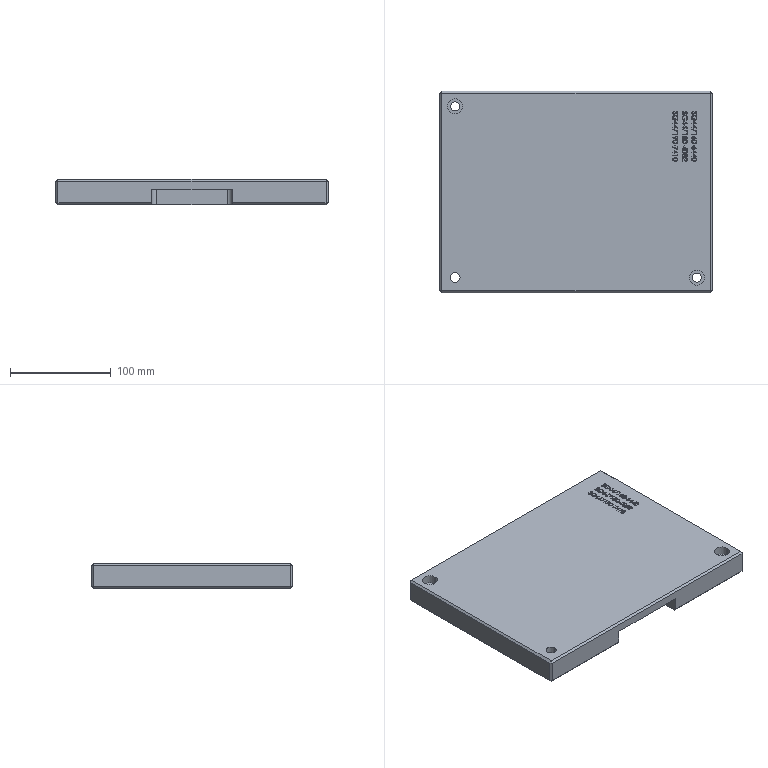Part | STEP file | Screw lock-base plate PN_0001 | 1 solid | 536 faces | box 270 x 200 x 25 mm | volume 1267432 mm3 | plane 323 | spline 193 | cylinder 14 | cone 6 | commonest cylinder face diameters 10 x6 9 x4 15 x4